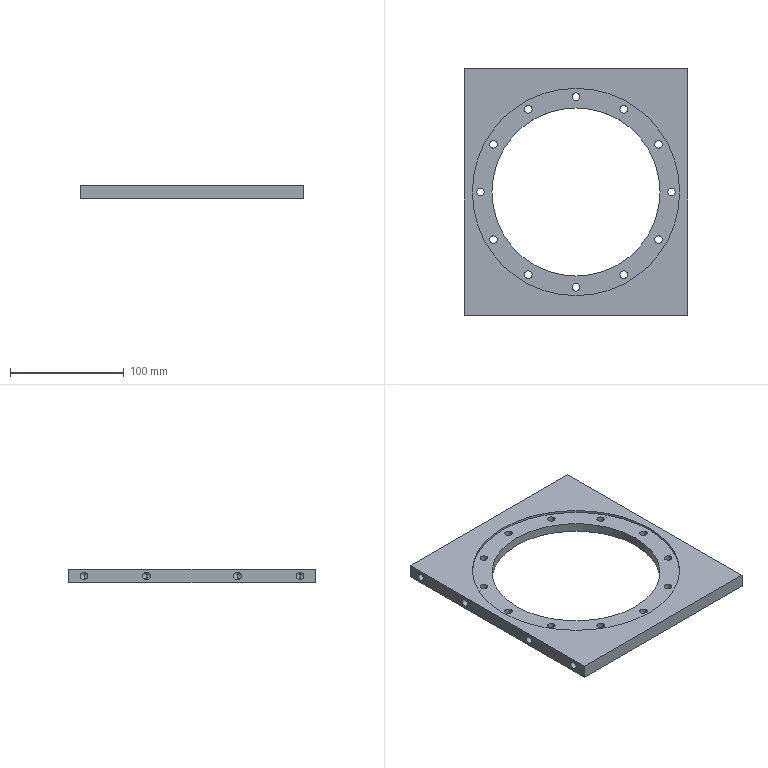Part | SolidWorks | features HoleWzd 3, ICE 2, Extrusion 1 | 1 solid | 70 faces | box 196.5 x 217 x 12 mm | volume 260204 mm3 | cylinder 46 | cone 16 | plane 8 | commonest cylinder face diameters 6.6 x24 6.8 x16 182.5 x4 148 x2